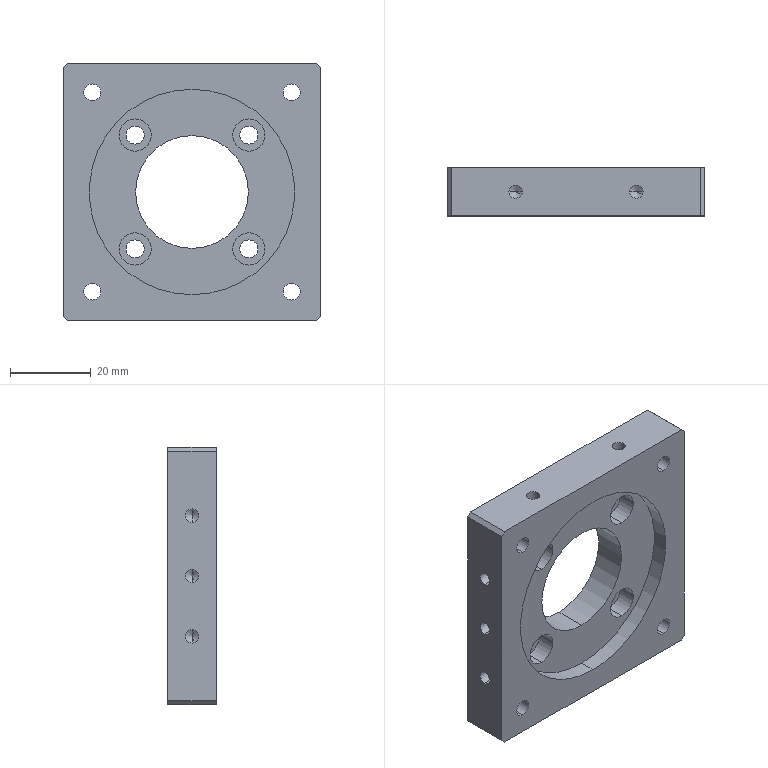Part | STEP file | Siemens 400W motor mounting plate | 1 solid | 83 faces | box 64 x 12 x 64 mm | volume 33213 mm3 | cylinder 48 | cone 20 | plane 15 | commonest cylinder face diameters 3.3 x20 4.2 x8 4.5 x8 8 x8 28 x2 51 x2